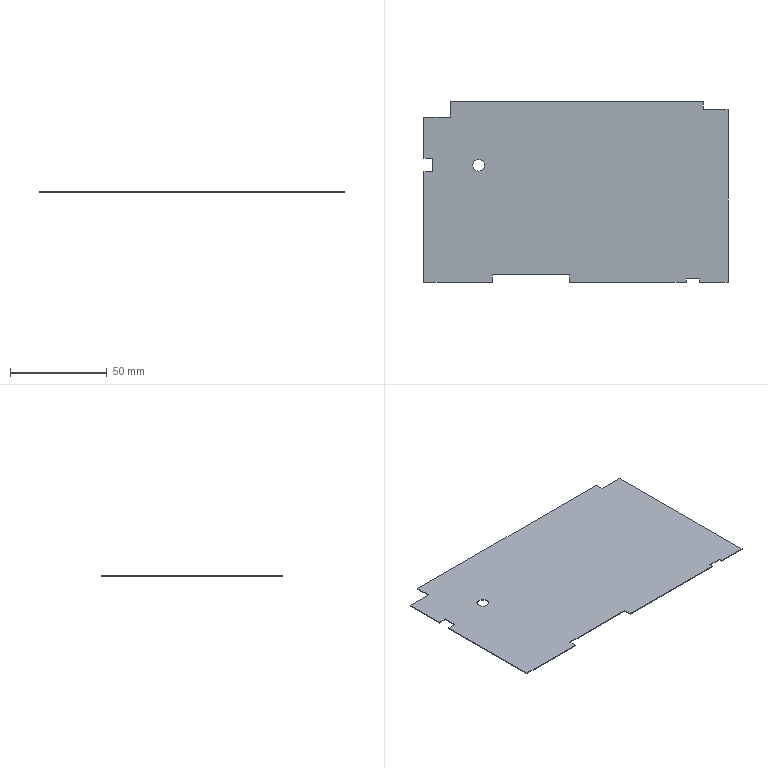Part | STEP file | LRS-150-12_X2_5F00517375-151329 | 1 solid | 24 faces | box 157 x 93.4 x 0.4 mm | volume 5710 mm3 | plane 22 | cylinder 2 | commonest cylinder face diameters 6 x2